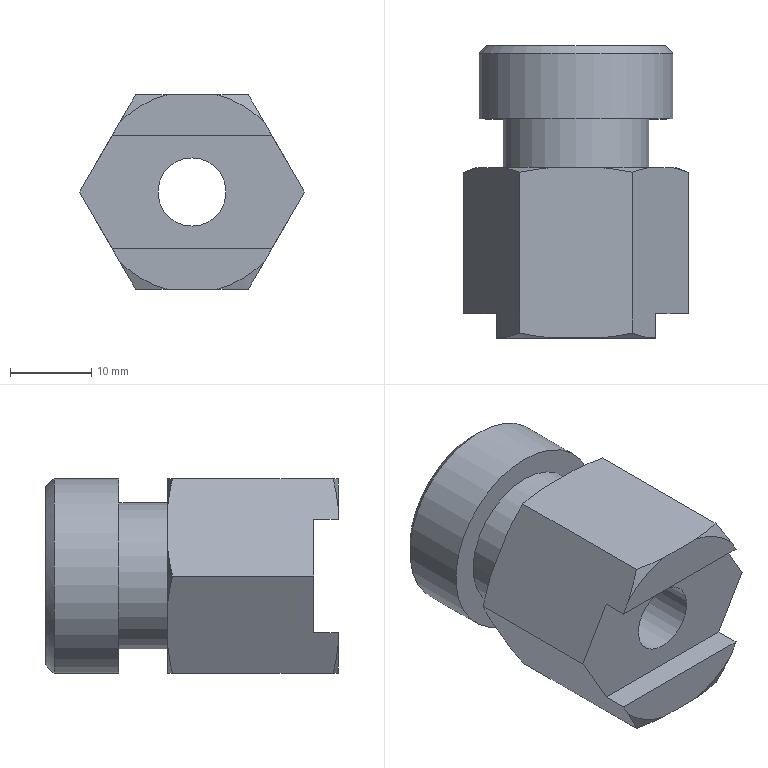Part | NX | 1 solid | 30 faces | box 27.713 x 36 x 24 mm | volume 12114 mm3 | plane 15 | cone 11 | cylinder 4 | commonest cylinder face diameters 8.4 x1 15 x1 18 x1 24 x1
STEP:
#1=CARTESIAN_POINT('',(6.928,-20.4,12.));
#2=VERTEX_POINT('',#1);
#3=CARTESIAN_POINT('',(6.928,-0.6,12.));
#4=VERTEX_POINT('',#3);
#5=CARTESIAN_POINT('',(6.928,-21.,12.));
#6=DIRECTION('',(0.,1.,0.));
#7=VECTOR('',#6,1000.);
#8=LINE('',#5,#7);
#9=EDGE_CURVE('',#2,#4,#8,.T.);
#10=ORIENTED_EDGE('',*,*,#9,.F.);
#11=CARTESIAN_POINT('',(8.919,-21.,8.552));
#12=VERTEX_POINT('',#11);
#13=CARTESIAN_POINT('',(6.928,-20.4,12.));
#14=CARTESIAN_POINT('',(7.585,-20.663,10.862));
#15=CARTESIAN_POINT('',(8.248,-20.872,9.715));
#16=CARTESIAN_POINT('',(8.919,-21.,8.552));
#17=B_SPLINE_CURVE_WITH_KNOTS('',3,(#13,#14,#15,#16),.UNSPECIFIED.,.F.,.F.,(4,4),(0.009948,0.01397),.UNSPECIFIED.);
#18=EDGE_CURVE('',#2,#12,#17,.T.);
#19=ORIENTED_EDGE('',*,*,#18,.T.);
#20=CARTESIAN_POINT('',(9.815,-21.,7.));
#21=VERTEX_POINT('',#20);
#22=CARTESIAN_POINT('',(6.928,-21.,12.));
#23=DIRECTION('',(0.5,0.,-0.866));
#24=VECTOR('',#23,1000.);
#25=LINE('',#22,#24);
#26=EDGE_CURVE('',#12,#21,#25,.T.);
#27=ORIENTED_EDGE('',*,*,#26,.T.);
#28=CARTESIAN_POINT('',(9.815,-18.,7.));
#29=VERTEX_POINT('',#28);
#30=CARTESIAN_POINT('',(9.815,-21.,7.));
#31=DIRECTION('',(0.,-1.,0.));
#32=VECTOR('',#31,1000.);
#33=LINE('',#30,#32);
#34=EDGE_CURVE('',#29,#21,#33,.T.);
#35=ORIENTED_EDGE('',*,*,#34,.F.);
#36=CARTESIAN_POINT('',(13.856,-18.,0.));
#37=VERTEX_POINT('',#36);
#38=CARTESIAN_POINT('',(6.928,-18.,12.));
#39=DIRECTION('',(-0.5,0.,0.866));
#40=VECTOR('',#39,1000.);
#41=LINE('',#38,#40);
#42=EDGE_CURVE('',#37,#29,#41,.T.);
#43=ORIENTED_EDGE('',*,*,#42,.F.);
#44=CARTESIAN_POINT('',(13.856,-0.6,0.));
#45=VERTEX_POINT('',#44);
#46=CARTESIAN_POINT('',(13.856,-21.,0.));
#47=DIRECTION('',(0.,1.,0.));
#48=VECTOR('',#47,1000.);
#49=LINE('',#46,#48);
#50=EDGE_CURVE('',#37,#45,#49,.T.);
#51=ORIENTED_EDGE('',*,*,#50,.T.);
#52=CARTESIAN_POINT('',(11.865,0.,3.448));
#53=VERTEX_POINT('',#52);
#54=CARTESIAN_POINT('',(13.856,-0.6,0.));
#55=CARTESIAN_POINT('',(13.2,-0.3373,1.138));
#56=CARTESIAN_POINT('',(12.537,-0.1281,2.285));
#57=CARTESIAN_POINT('',(11.865,0.,3.448));
#58=B_SPLINE_CURVE_WITH_KNOTS('',3,(#54,#55,#56,#57),.UNSPECIFIED.,.F.,.F.,(4,4),(0.009948,0.01397),.UNSPECIFIED.);
#59=EDGE_CURVE('',#45,#53,#58,.T.);
#60=ORIENTED_EDGE('',*,*,#59,.T.);
#61=CARTESIAN_POINT('',(8.919,0.,8.552));
#62=VERTEX_POINT('',#61);
#63=CARTESIAN_POINT('',(6.928,0.,12.));
#64=DIRECTION('',(0.5,0.,-0.866));
#65=VECTOR('',#64,1000.);
#66=LINE('',#63,#65);
#67=EDGE_CURVE('',#62,#53,#66,.T.);
#68=ORIENTED_EDGE('',*,*,#67,.F.);
#69=CARTESIAN_POINT('',(8.919,0.,8.552));
#70=CARTESIAN_POINT('',(8.249,-0.1279,9.713));
#71=CARTESIAN_POINT('',(7.586,-0.337,10.861));
#72=CARTESIAN_POINT('',(6.928,-0.6,12.));
#73=B_SPLINE_CURVE_WITH_KNOTS('',3,(#69,#70,#71,#72),.UNSPECIFIED.,.F.,.F.,(4,4),(0.01983,0.02389),.UNSPECIFIED.);
#74=EDGE_CURVE('',#62,#4,#73,.T.);
#75=ORIENTED_EDGE('',*,*,#74,.T.);
#76=EDGE_LOOP('',(#10,#19,#27,#35,#43,#51,#60,#68,#75));
#77=FACE_BOUND('',#76,.T.);
#78=CARTESIAN_POINT('',(6.928,-21.,12.));
#79=DIRECTION('',(0.866,0.,0.5));
#80=DIRECTION('',(0.5,0.,-0.866));
#81=AXIS2_PLACEMENT_3D('',#78,#79,#80);
#82=PLANE('',#81);
#83=ADVANCED_FACE('',(#77),#82,.T.);
#84=CARTESIAN_POINT('',(-6.928,-20.4,12.));
#85=VERTEX_POINT('',#84);
#86=CARTESIAN_POINT('',(-6.928,-0.6,12.));
#87=VERTEX_POINT('',#86);
#88=CARTESIAN_POINT('',(-6.928,-21.,12.));
#89=DIRECTION('',(0.,1.,0.));
#90=VECTOR('',#89,1000.);
#91=LINE('',#88,#90);
#92=EDGE_CURVE('',#85,#87,#91,.T.);
#93=ORIENTED_EDGE('',*,*,#92,.F.);
#94=CARTESIAN_POINT('',(-2.946,-21.,12.));
#95=VERTEX_POINT('',#94);
#96=CARTESIAN_POINT('',(-6.928,-20.4,12.));
#97=CARTESIAN_POINT('',(-5.613,-20.663,12.));
#98=CARTESIAN_POINT('',(-4.288,-20.872,12.));
#99=CARTESIAN_POINT('',(-2.946,-21.,12.));
#100=B_SPLINE_CURVE_WITH_KNOTS('',3,(#96,#97,#98,#99),.UNSPECIFIED.,.F.,.F.,(4,4),(0.008595,0.01262),.UNSPECIFIED.);
#101=EDGE_CURVE('',#85,#95,#100,.T.);
#102=ORIENTED_EDGE('',*,*,#101,.T.);
#103=CARTESIAN_POINT('',(2.946,-21.,12.));
#104=VERTEX_POINT('',#103);
#105=CARTESIAN_POINT('',(-6.928,-21.,12.));
#106=DIRECTION('',(1.,0.,0.));
#107=VECTOR('',#106,1000.);
#108=LINE('',#105,#107);
#109=EDGE_CURVE('',#95,#104,#108,.T.);
#110=ORIENTED_EDGE('',*,*,#109,.T.);
#111=CARTESIAN_POINT('',(2.946,-21.,12.));
#112=CARTESIAN_POINT('',(4.287,-20.872,12.));
#113=CARTESIAN_POINT('',(5.613,-20.663,12.));
#114=CARTESIAN_POINT('',(6.928,-20.4,12.));
#115=B_SPLINE_CURVE_WITH_KNOTS('',3,(#111,#112,#113,#114),.UNSPECIFIED.,.F.,.F.,(4,4),(0.01847,0.0225),.UNSPECIFIED.);
#116=EDGE_CURVE('',#104,#2,#115,.T.);
#117=ORIENTED_EDGE('',*,*,#116,.T.);
#118=ORIENTED_EDGE('',*,*,#9,.T.);
#119=CARTESIAN_POINT('',(2.946,0.,12.));
#120=VERTEX_POINT('',#119);
#121=CARTESIAN_POINT('',(6.928,-0.6,12.));
#122=CARTESIAN_POINT('',(5.613,-0.337,12.));
#123=CARTESIAN_POINT('',(4.288,-0.128,12.));
#124=CARTESIAN_POINT('',(2.946,0.,12.));
#125=B_SPLINE_CURVE_WITH_KNOTS('',3,(#121,#122,#123,#124),.UNSPECIFIED.,.F.,.F.,(4,4),(0.008595,0.01262),.UNSPECIFIED.);
#126=EDGE_CURVE('',#4,#120,#125,.T.);
#127=ORIENTED_EDGE('',*,*,#126,.T.);
#128=CARTESIAN_POINT('',(-2.946,0.,12.));
#129=VERTEX_POINT('',#128);
#130=CARTESIAN_POINT('',(-6.928,0.,12.));
#131=DIRECTION('',(1.,0.,0.));
#132=VECTOR('',#131,1000.);
#133=LINE('',#130,#132);
#134=EDGE_CURVE('',#129,#120,#133,.T.);
#135=ORIENTED_EDGE('',*,*,#134,.F.);
#136=CARTESIAN_POINT('',(-2.946,0.,12.));
#137=CARTESIAN_POINT('',(-4.287,-0.1279,12.));
#138=CARTESIAN_POINT('',(-5.613,-0.3369,12.));
#139=CARTESIAN_POINT('',(-6.928,-0.6,12.));
#140=B_SPLINE_CURVE_WITH_KNOTS('',3,(#136,#137,#138,#139),.UNSPECIFIED.,.F.,.F.,(4,4),(0.01847,0.0225),.UNSPECIFIED.);
#141=EDGE_CURVE('',#129,#87,#140,.T.);
#142=ORIENTED_EDGE('',*,*,#141,.T.);
#143=EDGE_LOOP('',(#93,#102,#110,#117,#118,#127,#135,#142));
#144=FACE_BOUND('',#143,.T.);
#145=CARTESIAN_POINT('',(-6.928,-21.,12.));
#146=DIRECTION('',(0.,0.,1.));
#147=DIRECTION('',(1.,0.,0.));
#148=AXIS2_PLACEMENT_3D('',#145,#146,#147);
#149=PLANE('',#148);
#150=ADVANCED_FACE('',(#144),#149,.T.);
#151=CARTESIAN_POINT('',(-9.815,-21.,7.));
#152=VERTEX_POINT('',#151);
#153=CARTESIAN_POINT('',(-8.919,-21.,8.552));
#154=VERTEX_POINT('',#153);
#155=CARTESIAN_POINT('',(-13.856,-21.,0.));
#156=DIRECTION('',(0.5,0.,0.866));
#157=VECTOR('',#156,1000.);
#158=LINE('',#155,#157);
#159=EDGE_CURVE('',#152,#154,#158,.T.);
#160=ORIENTED_EDGE('',*,*,#159,.T.);
#161=CARTESIAN_POINT('',(-8.919,-21.,8.552));
#162=CARTESIAN_POINT('',(-8.249,-20.872,9.713));
#163=CARTESIAN_POINT('',(-7.586,-20.663,10.861));
#164=CARTESIAN_POINT('',(-6.928,-20.4,12.));
#165=B_SPLINE_CURVE_WITH_KNOTS('',3,(#161,#162,#163,#164),.UNSPECIFIED.,.F.,.F.,(4,4),(0.01983,0.02389),.UNSPECIFIED.);
#166=EDGE_CURVE('',#154,#85,#165,.T.);
#167=ORIENTED_EDGE('',*,*,#166,.T.);
#168=ORIENTED_EDGE('',*,*,#92,.T.);
#169=CARTESIAN_POINT('',(-8.919,0.,8.552));
#170=VERTEX_POINT('',#169);
#171=CARTESIAN_POINT('',(-6.928,-0.6,12.));
#172=CARTESIAN_POINT('',(-7.585,-0.3373,10.862));
#173=CARTESIAN_POINT('',(-8.248,-0.1281,9.715));
#174=CARTESIAN_POINT('',(-8.919,0.,8.552));
#175=B_SPLINE_CURVE_WITH_KNOTS('',3,(#171,#172,#173,#174),.UNSPECIFIED.,.F.,.F.,(4,4),(0.009948,0.01397),.UNSPECIFIED.);
#176=EDGE_CURVE('',#87,#170,#175,.T.);
#177=ORIENTED_EDGE('',*,*,#176,.T.);
#178=CARTESIAN_POINT('',(-11.865,0.,3.448));
#179=VERTEX_POINT('',#178);
#180=CARTESIAN_POINT('',(-13.856,0.,0.));
#181=DIRECTION('',(0.5,0.,0.866));
#182=VECTOR('',#181,1000.);
#183=LINE('',#180,#182);
#184=EDGE_CURVE('',#179,#170,#183,.T.);
#185=ORIENTED_EDGE('',*,*,#184,.F.);
#186=CARTESIAN_POINT('',(-13.856,-0.6,0.));
#187=VERTEX_POINT('',#186);
#188=CARTESIAN_POINT('',(-11.865,0.,3.448));
#189=CARTESIAN_POINT('',(-12.536,-0.1279,2.287));
#190=CARTESIAN_POINT('',(-13.199,-0.337,1.139));
#191=CARTESIAN_POINT('',(-13.856,-0.6,0.));
#192=B_SPLINE_CURVE_WITH_KNOTS('',3,(#188,#189,#190,#191),.UNSPECIFIED.,.F.,.F.,(4,4),(0.01983,0.02389),.UNSPECIFIED.);
#193=EDGE_CURVE('',#179,#187,#192,.T.);
#194=ORIENTED_EDGE('',*,*,#193,.T.);
#195=CARTESIAN_POINT('',(-13.856,-18.,0.));
#196=VERTEX_POINT('',#195);
#197=CARTESIAN_POINT('',(-13.856,-21.,0.));
#198=DIRECTION('',(0.,1.,0.));
#199=VECTOR('',#198,1000.);
#200=LINE('',#197,#199);
#201=EDGE_CURVE('',#196,#187,#200,.T.);
#202=ORIENTED_EDGE('',*,*,#201,.F.);
#203=CARTESIAN_POINT('',(-9.815,-18.,7.));
#204=VERTEX_POINT('',#203);
#205=CARTESIAN_POINT('',(-13.856,-18.,0.));
#206=DIRECTION('',(-0.5,0.,-0.866));
#207=VECTOR('',#206,1000.);
#208=LINE('',#205,#207);
#209=EDGE_CURVE('',#204,#196,#208,.T.);
#210=ORIENTED_EDGE('',*,*,#209,.F.);
#211=CARTESIAN_POINT('',(-9.815,-21.,7.));
#212=DIRECTION('',(0.,1.,0.));
#213=VECTOR('',#212,1000.);
#214=LINE('',#211,#213);
#215=EDGE_CURVE('',#152,#204,#214,.T.);
#216=ORIENTED_EDGE('',*,*,#215,.F.);
#217=EDGE_LOOP('',(#160,#167,#168,#177,#185,#194,#202,#210,#216));
#218=FACE_BOUND('',#217,.T.);
#219=CARTESIAN_POINT('',(-13.856,-21.,0.));
#220=DIRECTION('',(-0.866,0.,0.5));
#221=DIRECTION('',(0.5,0.,0.866));
#222=AXIS2_PLACEMENT_3D('',#219,#220,#221);
#223=PLANE('',#222);
#224=ADVANCED_FACE('',(#218),#223,.T.);
#225=CARTESIAN_POINT('',(-6.928,-20.4,-12.));
#226=VERTEX_POINT('',#225);
#227=CARTESIAN_POINT('',(-6.928,-0.6,-12.));
#228=VERTEX_POINT('',#227);
#229=CARTESIAN_POINT('',(-6.928,-21.,-12.));
#230=DIRECTION('',(0.,1.,0.));
#231=VECTOR('',#230,1000.);
#232=LINE('',#229,#231);
#233=EDGE_CURVE('',#226,#228,#232,.T.);
#234=ORIENTED_EDGE('',*,*,#233,.F.);
#235=CARTESIAN_POINT('',(-8.919,-21.,-8.552));
#236=VERTEX_POINT('',#235);
#237=CARTESIAN_POINT('',(-6.928,-20.4,-12.));
#238=CARTESIAN_POINT('',(-7.585,-20.663,-10.862));
#239=CARTESIAN_POINT('',(-8.248,-20.872,-9.715));
#240=CARTESIAN_POINT('',(-8.919,-21.,-8.552));
#241=B_SPLINE_CURVE_WITH_KNOTS('',3,(#237,#238,#239,#240),.UNSPECIFIED.,.F.,.F.,(4,4),(0.009948,0.01397),.UNSPECIFIED.);
#242=EDGE_CURVE('',#226,#236,#241,.T.);
#243=ORIENTED_EDGE('',*,*,#242,.T.);
#244=CARTESIAN_POINT('',(-9.815,-21.,-7.));
#245=VERTEX_POINT('',#244);
#246=CARTESIAN_POINT('',(-6.928,-21.,-12.));
#247=DIRECTION('',(-0.5,0.,0.866));
#248=VECTOR('',#247,1000.);
#249=LINE('',#246,#248);
#250=EDGE_CURVE('',#236,#245,#249,.T.);
#251=ORIENTED_EDGE('',*,*,#250,.T.);
#252=CARTESIAN_POINT('',(-9.815,-18.,-7.));
#253=VERTEX_POINT('',#252);
#254=CARTESIAN_POINT('',(-9.815,-21.,-7.));
#255=DIRECTION('',(0.,-1.,0.));
#256=VECTOR('',#255,1000.);
#257=LINE('',#254,#256);
#258=EDGE_CURVE('',#253,#245,#257,.T.);
#259=ORIENTED_EDGE('',*,*,#258,.F.);
#260=CARTESIAN_POINT('',(-6.928,-18.,-12.));
#261=DIRECTION('',(0.5,0.,-0.866));
#262=VECTOR('',#261,1000.);
#263=LINE('',#260,#262);
#264=EDGE_CURVE('',#196,#253,#263,.T.);
#265=ORIENTED_EDGE('',*,*,#264,.F.);
#266=ORIENTED_EDGE('',*,*,#201,.T.);
#267=CARTESIAN_POINT('',(-11.865,0.,-3.448));
#268=VERTEX_POINT('',#267);
#269=CARTESIAN_POINT('',(-13.856,-0.6,0.));
#270=CARTESIAN_POINT('',(-13.2,-0.3373,-1.138));
#271=CARTESIAN_POINT('',(-12.537,-0.1281,-2.285));
#272=CARTESIAN_POINT('',(-11.865,0.,-3.448));
#273=B_SPLINE_CURVE_WITH_KNOTS('',3,(#269,#270,#271,#272),.UNSPECIFIED.,.F.,.F.,(4,4),(0.009948,0.01397),.UNSPECIFIED.);
#274=EDGE_CURVE('',#187,#268,#273,.T.);
#275=ORIENTED_EDGE('',*,*,#274,.T.);
#276=CARTESIAN_POINT('',(-8.919,0.,-8.552));
#277=VERTEX_POINT('',#276);
#278=CARTESIAN_POINT('',(-6.928,0.,-12.));
#279=DIRECTION('',(-0.5,0.,0.866));
#280=VECTOR('',#279,1000.);
#281=LINE('',#278,#280);
#282=EDGE_CURVE('',#277,#268,#281,.T.);
#283=ORIENTED_EDGE('',*,*,#282,.F.);
#284=CARTESIAN_POINT('',(-8.919,0.,-8.552));
#285=CARTESIAN_POINT('',(-8.249,-0.1279,-9.713));
#286=CARTESIAN_POINT('',(-7.586,-0.337,-10.861));
#287=CARTESIAN_POINT('',(-6.928,-0.6,-12.));
#288=B_SPLINE_CURVE_WITH_KNOTS('',3,(#284,#285,#286,#287),.UNSPECIFIED.,.F.,.F.,(4,4),(0.01983,0.02389),.UNSPECIFIED.);
#289=EDGE_CURVE('',#277,#228,#288,.T.);
#290=ORIENTED_EDGE('',*,*,#289,.T.);
#291=EDGE_LOOP('',(#234,#243,#251,#259,#265,#266,#275,#283,#290));
#292=FACE_BOUND('',#291,.T.);
#293=CARTESIAN_POINT('',(-6.928,-21.,-12.));
#294=DIRECTION('',(-0.866,0.,-0.5));
#295=DIRECTION('',(-0.5,0.,0.866));
#296=AXIS2_PLACEMENT_3D('',#293,#294,#295);
#297=PLANE('',#296);
#298=ADVANCED_FACE('',(#292),#297,.T.);
#299=CARTESIAN_POINT('',(6.928,-20.4,-12.));
#300=VERTEX_POINT('',#299);
#301=CARTESIAN_POINT('',(6.928,-0.6,-12.));
#302=VERTEX_POINT('',#301);
#303=CARTESIAN_POINT('',(6.928,-21.,-12.));
#304=DIRECTION('',(0.,1.,0.));
#305=VECTOR('',#304,1000.);
#306=LINE('',#303,#305);
#307=EDGE_CURVE('',#300,#302,#306,.T.);
#308=ORIENTED_EDGE('',*,*,#307,.F.);
#309=CARTESIAN_POINT('',(2.946,-21.,-12.));
#310=VERTEX_POINT('',#309);
#311=CARTESIAN_POINT('',(6.928,-20.4,-12.));
#312=CARTESIAN_POINT('',(5.613,-20.663,-12.));
#313=CARTESIAN_POINT('',(4.288,-20.872,-12.));
#314=CARTESIAN_POINT('',(2.946,-21.,-12.));
#315=B_SPLINE_CURVE_WITH_KNOTS('',3,(#311,#312,#313,#314),.UNSPECIFIED.,.F.,.F.,(4,4),(0.008595,0.01262),.UNSPECIFIED.);
#316=EDGE_CURVE('',#300,#310,#315,.T.);
#317=ORIENTED_EDGE('',*,*,#316,.T.);
#318=CARTESIAN_POINT('',(-2.946,-21.,-12.));
#319=VERTEX_POINT('',#318);
#320=CARTESIAN_POINT('',(6.928,-21.,-12.));
#321=DIRECTION('',(-1.,0.,0.));
#322=VECTOR('',#321,1000.);
#323=LINE('',#320,#322);
#324=EDGE_CURVE('',#310,#319,#323,.T.);
#325=ORIENTED_EDGE('',*,*,#324,.T.);
#326=CARTESIAN_POINT('',(-2.946,-21.,-12.));
#327=CARTESIAN_POINT('',(-4.287,-20.872,-12.));
#328=CARTESIAN_POINT('',(-5.613,-20.663,-12.));
#329=CARTESIAN_POINT('',(-6.928,-20.4,-12.));
#330=B_SPLINE_CURVE_WITH_KNOTS('',3,(#326,#327,#328,#329),.UNSPECIFIED.,.F.,.F.,(4,4),(0.01847,0.0225),.UNSPECIFIED.);
#331=EDGE_CURVE('',#319,#226,#330,.T.);
#332=ORIENTED_EDGE('',*,*,#331,.T.);
#333=ORIENTED_EDGE('',*,*,#233,.T.);
#334=CARTESIAN_POINT('',(-2.946,0.,-12.));
#335=VERTEX_POINT('',#334);
#336=CARTESIAN_POINT('',(-6.928,-0.6,-12.));
#337=CARTESIAN_POINT('',(-5.613,-0.337,-12.));
#338=CARTESIAN_POINT('',(-4.288,-0.128,-12.));
#339=CARTESIAN_POINT('',(-2.946,0.,-12.));
#340=B_SPLINE_CURVE_WITH_KNOTS('',3,(#336,#337,#338,#339),.UNSPECIFIED.,.F.,.F.,(4,4),(0.008595,0.01262),.UNSPECIFIED.);
#341=EDGE_CURVE('',#228,#335,#340,.T.);
#342=ORIENTED_EDGE('',*,*,#341,.T.);
#343=CARTESIAN_POINT('',(2.946,0.,-12.));
#344=VERTEX_POINT('',#343);
#345=CARTESIAN_POINT('',(6.928,0.,-12.));
#346=DIRECTION('',(-1.,0.,0.));
#347=VECTOR('',#346,1000.);
#348=LINE('',#345,#347);
#349=EDGE_CURVE('',#344,#335,#348,.T.);
#350=ORIENTED_EDGE('',*,*,#349,.F.);
#351=CARTESIAN_POINT('',(2.946,0.,-12.));
#352=CARTESIAN_POINT('',(4.287,-0.1279,-12.));
#353=CARTESIAN_POINT('',(5.613,-0.3369,-12.));
#354=CARTESIAN_POINT('',(6.928,-0.6,-12.));
#355=B_SPLINE_CURVE_WITH_KNOTS('',3,(#351,#352,#353,#354),.UNSPECIFIED.,.F.,.F.,(4,4),(0.01847,0.0225),.UNSPECIFIED.);
#356=EDGE_CURVE('',#344,#302,#355,.T.);
#357=ORIENTED_EDGE('',*,*,#356,.T.);
#358=EDGE_LOOP('',(#308,#317,#325,#332,#333,#342,#350,#357));
#359=FACE_BOUND('',#358,.T.);
#360=CARTESIAN_POINT('',(6.928,-21.,-12.));
#361=DIRECTION('',(0.,0.,-1.));
#362=DIRECTION('',(-1.,0.,0.));
#363=AXIS2_PLACEMENT_3D('',#360,#361,#362);
#364=PLANE('',#363);
#365=ADVANCED_FACE('',(#359),#364,.T.);
#366=CARTESIAN_POINT('',(9.815,-21.,-7.));
#367=VERTEX_POINT('',#366);
#368=CARTESIAN_POINT('',(8.919,-21.,-8.552));
#369=VERTEX_POINT('',#368);
#370=CARTESIAN_POINT('',(13.856,-21.,0.));
#371=DIRECTION('',(-0.5,0.,-0.866));
#372=VECTOR('',#371,1000.);
#373=LINE('',#370,#372);
#374=EDGE_CURVE('',#367,#369,#373,.T.);
#375=ORIENTED_EDGE('',*,*,#374,.T.);
#376=CARTESIAN_POINT('',(8.919,-21.,-8.552));
#377=CARTESIAN_POINT('',(8.249,-20.872,-9.713));
#378=CARTESIAN_POINT('',(7.586,-20.663,-10.861));
#379=CARTESIAN_POINT('',(6.928,-20.4,-12.));
#380=B_SPLINE_CURVE_WITH_KNOTS('',3,(#376,#377,#378,#379),.UNSPECIFIED.,.F.,.F.,(4,4),(0.01983,0.02389),.UNSPECIFIED.);
#381=EDGE_CURVE('',#369,#300,#380,.T.);
#382=ORIENTED_EDGE('',*,*,#381,.T.);
#383=ORIENTED_EDGE('',*,*,#307,.T.);
#384=CARTESIAN_POINT('',(8.919,0.,-8.552));
#385=VERTEX_POINT('',#384);
#386=CARTESIAN_POINT('',(6.928,-0.6,-12.));
#387=CARTESIAN_POINT('',(7.585,-0.3373,-10.862));
#388=CARTESIAN_POINT('',(8.248,-0.1281,-9.715));
#389=CARTESIAN_POINT('',(8.919,0.,-8.552));
#390=B_SPLINE_CURVE_WITH_KNOTS('',3,(#386,#387,#388,#389),.UNSPECIFIED.,.F.,.F.,(4,4),(0.009948,0.01397),.UNSPECIFIED.);
#391=EDGE_CURVE('',#302,#385,#390,.T.);
#392=ORIENTED_EDGE('',*,*,#391,.T.);
#393=CARTESIAN_POINT('',(11.865,0.,-3.448));
#394=VERTEX_POINT('',#393);
#395=CARTESIAN_POINT('',(13.856,0.,0.));
#396=DIRECTION('',(-0.5,0.,-0.866));
#397=VECTOR('',#396,1000.);
#398=LINE('',#395,#397);
#399=EDGE_CURVE('',#394,#385,#398,.T.);
#400=ORIENTED_EDGE('',*,*,#399,.F.);
#401=CARTESIAN_POINT('',(11.865,0.,-3.448));
#402=CARTESIAN_POINT('',(12.536,-0.1279,-2.287));
#403=CARTESIAN_POINT('',(13.199,-0.337,-1.139));
#404=CARTESIAN_POINT('',(13.856,-0.6,0.));
#405=B_SPLINE_CURVE_WITH_KNOTS('',3,(#401,#402,#403,#404),.UNSPECIFIED.,.F.,.F.,(4,4),(0.01983,0.02389),.UNSPECIFIED.);
#406=EDGE_CURVE('',#394,#45,#405,.T.);
#407=ORIENTED_EDGE('',*,*,#406,.T.);
#408=ORIENTED_EDGE('',*,*,#50,.F.);
#409=CARTESIAN_POINT('',(9.815,-18.,-7.));
#410=VERTEX_POINT('',#409);
#411=CARTESIAN_POINT('',(13.856,-18.,0.));
#412=DIRECTION('',(0.5,0.,0.866));
#413=VECTOR('',#412,1000.);
#414=LINE('',#411,#413);
#415=EDGE_CURVE('',#410,#37,#414,.T.);
#416=ORIENTED_EDGE('',*,*,#415,.F.);
#417=CARTESIAN_POINT('',(9.815,-21.,-7.));
#418=DIRECTION('',(0.,1.,0.));
#419=VECTOR('',#418,1000.);
#420=LINE('',#417,#419);
#421=EDGE_CURVE('',#367,#410,#420,.T.);
#422=ORIENTED_EDGE('',*,*,#421,.F.);
#423=EDGE_LOOP('',(#375,#382,#383,#392,#400,#407,#408,#416,#422));
#424=FACE_BOUND('',#423,.T.);
#425=CARTESIAN_POINT('',(13.856,-21.,0.));
#426=DIRECTION('',(0.866,0.,-0.5));
#427=DIRECTION('',(-0.5,0.,-0.866));
#428=AXIS2_PLACEMENT_3D('',#425,#426,#427);
#429=PLANE('',#428);
#430=ADVANCED_FACE('',(#424),#429,.T.);
#431=CARTESIAN_POINT('',(0.,-21.,0.));
#432=DIRECTION('',(0.,1.,0.));
#433=DIRECTION('',(0.,0.,1.));
#434=AXIS2_PLACEMENT_3D('',#431,#432,#433);
#435=CIRCLE('',#434,12.356);
#436=EDGE_CURVE('',#104,#12,#435,.T.);
#437=ORIENTED_EDGE('',*,*,#436,.F.);
#438=ORIENTED_EDGE('',*,*,#109,.F.);
#439=CARTESIAN_POINT('',(0.,-21.,0.));
#440=DIRECTION('',(0.,1.,0.));
#441=DIRECTION('',(0.,0.,1.));
#442=AXIS2_PLACEMENT_3D('',#439,#440,#441);
#443=CIRCLE('',#442,12.356);
#444=EDGE_CURVE('',#154,#95,#443,.T.);
#445=ORIENTED_EDGE('',*,*,#444,.F.);
#446=ORIENTED_EDGE('',*,*,#159,.F.);
#447=CARTESIAN_POINT('',(0.,-21.,7.));
#448=DIRECTION('',(1.,0.,0.));
#449=VECTOR('',#448,1000.);
#450=LINE('',#447,#449);
#451=EDGE_CURVE('',#152,#21,#450,.T.);
#452=ORIENTED_EDGE('',*,*,#451,.T.);
#453=ORIENTED_EDGE('',*,*,#26,.F.);
#454=EDGE_LOOP('',(#437,#438,#445,#446,#452,#453));
#455=FACE_BOUND('',#454,.T.);
#456=CARTESIAN_POINT('',(0.,-21.,0.));
#457=DIRECTION('',(0.,1.,0.));
#458=DIRECTION('',(0.,0.,1.));
#459=AXIS2_PLACEMENT_3D('',#456,#457,#458);
#460=PLANE('',#459);
#461=ADVANCED_FACE('',(#455),#460,.F.);
#462=CARTESIAN_POINT('',(0.,-21.,0.));
#463=DIRECTION('',(0.,1.,0.));
#464=DIRECTION('',(0.,0.,1.));
#465=AXIS2_PLACEMENT_3D('',#462,#463,#464);
#466=CIRCLE('',#465,12.356);
#467=EDGE_CURVE('',#369,#310,#466,.T.);
#468=ORIENTED_EDGE('',*,*,#467,.F.);
#469=ORIENTED_EDGE('',*,*,#374,.F.);
#470=CARTESIAN_POINT('',(0.,-21.,-7.));
#471=DIRECTION('',(-1.,0.,0.));
#472=VECTOR('',#471,1000.);
#473=LINE('',#470,#472);
#474=EDGE_CURVE('',#367,#245,#473,.T.);
#475=ORIENTED_EDGE('',*,*,#474,.T.);
#476=ORIENTED_EDGE('',*,*,#250,.F.);
#477=CARTESIAN_POINT('',(0.,-21.,0.));
#478=DIRECTION('',(0.,1.,0.));
#479=DIRECTION('',(0.,0.,1.));
#480=AXIS2_PLACEMENT_3D('',#477,#478,#479);
#481=CIRCLE('',#480,12.356);
#482=EDGE_CURVE('',#319,#236,#481,.T.);
#483=ORIENTED_EDGE('',*,*,#482,.F.);
#484=ORIENTED_EDGE('',*,*,#324,.F.);
#485=EDGE_LOOP('',(#468,#469,#475,#476,#483,#484));
#486=FACE_BOUND('',#485,.T.);
#487=CARTESIAN_POINT('',(0.,-21.,0.));
#488=DIRECTION('',(0.,1.,0.));
#489=DIRECTION('',(0.,0.,1.));
#490=AXIS2_PLACEMENT_3D('',#487,#488,#489);
#491=PLANE('',#490);
#492=ADVANCED_FACE('',(#486),#491,.F.);
#493=CARTESIAN_POINT('',(0.,0.,9.));
#494=VERTEX_POINT('',#493);
#495=CARTESIAN_POINT('',(0.,0.,0.));
#496=DIRECTION('',(0.,1.,0.));
#497=DIRECTION('',(0.,0.,1.));
#498=AXIS2_PLACEMENT_3D('',#495,#496,#497);
#499=CIRCLE('',#498,9.);
#500=EDGE_CURVE('',#494,#494,#499,.T.);
#501=ORIENTED_EDGE('',*,*,#500,.F.);
#502=EDGE_LOOP('',(#501));
#503=FACE_BOUND('',#502,.T.);
#504=ORIENTED_EDGE('',*,*,#134,.T.);
#505=CARTESIAN_POINT('',(0.,0.,0.));
#506=DIRECTION('',(0.,1.,0.));
#507=DIRECTION('',(0.,0.,1.));
#508=AXIS2_PLACEMENT_3D('',#505,#506,#507);
#509=CIRCLE('',#508,12.356);
#510=EDGE_CURVE('',#120,#62,#509,.T.);
#511=ORIENTED_EDGE('',*,*,#510,.T.);
#512=ORIENTED_EDGE('',*,*,#67,.T.);
#513=CARTESIAN_POINT('',(0.,0.,0.));
#514=DIRECTION('',(0.,1.,0.));
#515=DIRECTION('',(0.,0.,1.));
#516=AXIS2_PLACEMENT_3D('',#513,#514,#515);
#517=CIRCLE('',#516,12.356);
#518=EDGE_CURVE('',#53,#394,#517,.T.);
#519=ORIENTED_EDGE('',*,*,#518,.T.);
#520=ORIENTED_EDGE('',*,*,#399,.T.);
#521=CARTESIAN_POINT('',(0.,0.,0.));
#522=DIRECTION('',(0.,1.,0.));
#523=DIRECTION('',(0.,0.,1.));
#524=AXIS2_PLACEMENT_3D('',#521,#522,#523);
#525=CIRCLE('',#524,12.356);
#526=EDGE_CURVE('',#385,#344,#525,.T.);
#527=ORIENTED_EDGE('',*,*,#526,.T.);
#528=ORIENTED_EDGE('',*,*,#349,.T.);
#529=CARTESIAN_POINT('',(0.,0.,0.));
#530=DIRECTION('',(0.,1.,0.));
#531=DIRECTION('',(0.,0.,1.));
#532=AXIS2_PLACEMENT_3D('',#529,#530,#531);
#533=CIRCLE('',#532,12.356);
#534=EDGE_CURVE('',#335,#277,#533,.T.);
#535=ORIENTED_EDGE('',*,*,#534,.T.);
#536=ORIENTED_EDGE('',*,*,#282,.T.);
#537=CARTESIAN_POINT('',(0.,0.,0.));
#538=DIRECTION('',(0.,1.,0.));
#539=DIRECTION('',(0.,0.,1.));
#540=AXIS2_PLACEMENT_3D('',#537,#538,#539);
#541=CIRCLE('',#540,12.356);
#542=EDGE_CURVE('',#268,#179,#541,.T.);
#543=ORIENTED_EDGE('',*,*,#542,.T.);
#544=ORIENTED_EDGE('',*,*,#184,.T.);
#545=CARTESIAN_POINT('',(0.,0.,0.));
#546=DIRECTION('',(0.,1.,0.));
#547=DIRECTION('',(0.,0.,1.));
#548=AXIS2_PLACEMENT_3D('',#545,#546,#547);
#549=CIRCLE('',#548,12.356);
#550=EDGE_CURVE('',#170,#129,#549,.T.);
#551=ORIENTED_EDGE('',*,*,#550,.T.);
#552=EDGE_LOOP('',(#504,#511,#512,#519,#520,#527,#528,#535,#536,#543,#544,#551));
#553=FACE_BOUND('',#552,.T.);
#554=CARTESIAN_POINT('',(0.,0.,0.));
#555=DIRECTION('',(0.,1.,0.));
#556=DIRECTION('',(0.,0.,1.));
#557=AXIS2_PLACEMENT_3D('',#554,#555,#556);
#558=PLANE('',#557);
#559=ADVANCED_FACE('',(#503,#553),#558,.T.);
#560=CARTESIAN_POINT('',(0.,6.,9.));
#561=VERTEX_POINT('',#560);
#562=CARTESIAN_POINT('',(0.,6.,0.));
#563=DIRECTION('',(0.,1.,0.));
#564=DIRECTION('',(0.,0.,1.));
#565=AXIS2_PLACEMENT_3D('',#562,#563,#564);
#566=CIRCLE('',#565,9.);
#567=EDGE_CURVE('',#561,#561,#566,.T.);
#568=ORIENTED_EDGE('',*,*,#567,.T.);
#569=EDGE_LOOP('',(#568));
#570=FACE_BOUND('',#569,.T.);
#571=CARTESIAN_POINT('',(0.,6.,12.));
#572=VERTEX_POINT('',#571);
#573=CARTESIAN_POINT('',(0.,6.,0.));
#574=DIRECTION('',(0.,1.,0.));
#575=DIRECTION('',(0.,0.,1.));
#576=AXIS2_PLACEMENT_3D('',#573,#574,#575);
#577=CIRCLE('',#576,12.);
#578=EDGE_CURVE('',#572,#572,#577,.T.);
#579=ORIENTED_EDGE('',*,*,#578,.F.);
#580=EDGE_LOOP('',(#579));
#581=FACE_BOUND('',#580,.T.);
#582=CARTESIAN_POINT('',(0.,6.,0.));
#583=DIRECTION('',(0.,1.,0.));
#584=DIRECTION('',(0.,0.,1.));
#585=AXIS2_PLACEMENT_3D('',#582,#583,#584);
#586=PLANE('',#585);
#587=ADVANCED_FACE('',(#570,#581),#586,.F.);
#588=CARTESIAN_POINT('',(0.,15.,11.));
#589=VERTEX_POINT('',#588);
#590=CARTESIAN_POINT('',(0.,15.,0.));
#591=DIRECTION('',(0.,1.,0.));
#592=DIRECTION('',(0.,0.,1.));
#593=AXIS2_PLACEMENT_3D('',#590,#591,#592);
#594=CIRCLE('',#593,11.);
#595=EDGE_CURVE('',#589,#589,#594,.T.);
#596=ORIENTED_EDGE('',*,*,#595,.T.);
#597=EDGE_LOOP('',(#596));
#598=FACE_BOUND('',#597,.T.);
#599=CARTESIAN_POINT('',(0.,15.,7.5));
#600=VERTEX_POINT('',#599);
#601=CARTESIAN_POINT('',(0.,15.,0.));
#602=DIRECTION('',(0.,1.,0.));
#603=DIRECTION('',(0.,0.,1.));
#604=AXIS2_PLACEMENT_3D('',#601,#602,#603);
#605=CIRCLE('',#604,7.5);
#606=EDGE_CURVE('',#600,#600,#605,.T.);
#607=ORIENTED_EDGE('',*,*,#606,.F.);
#608=EDGE_LOOP('',(#607));
#609=FACE_BOUND('',#608,.T.);
#610=CARTESIAN_POINT('',(0.,15.,0.));
#611=DIRECTION('',(0.,1.,0.));
#612=DIRECTION('',(0.,0.,1.));
#613=AXIS2_PLACEMENT_3D('',#610,#611,#612);
#614=PLANE('',#613);
#615=ADVANCED_FACE('',(#598,#609),#614,.T.);
#616=ORIENTED_EDGE('',*,*,#34,.T.);
#617=ORIENTED_EDGE('',*,*,#451,.F.);
#618=ORIENTED_EDGE('',*,*,#215,.T.);
#619=CARTESIAN_POINT('',(-15.,-18.,7.));
#620=DIRECTION('',(-1.,0.,0.));
#621=VECTOR('',#620,1000.);
#622=LINE('',#619,#621);
#623=EDGE_CURVE('',#29,#204,#622,.T.);
#624=ORIENTED_EDGE('',*,*,#623,.F.);
#625=EDGE_LOOP('',(#616,#617,#618,#624));
#626=FACE_BOUND('',#625,.T.);
#627=CARTESIAN_POINT('',(-15.,-18.,7.));
#628=DIRECTION('',(0.,0.,1.));
#629=DIRECTION('',(1.,0.,0.));
#630=AXIS2_PLACEMENT_3D('',#627,#628,#629);
#631=PLANE('',#630);
#632=ADVANCED_FACE('',(#626),#631,.F.);
#633=ORIENTED_EDGE('',*,*,#258,.T.);
#634=ORIENTED_EDGE('',*,*,#474,.F.);
#635=ORIENTED_EDGE('',*,*,#421,.T.);
#636=CARTESIAN_POINT('',(-15.,-18.,-7.));
#637=DIRECTION('',(1.,0.,0.));
#638=VECTOR('',#637,1000.);
#639=LINE('',#636,#638);
#640=EDGE_CURVE('',#253,#410,#639,.T.);
#641=ORIENTED_EDGE('',*,*,#640,.F.);
#642=EDGE_LOOP('',(#633,#634,#635,#641));
#643=FACE_BOUND('',#642,.T.);
#644=CARTESIAN_POINT('',(-15.,-18.,-7.));
#645=DIRECTION('',(0.,0.,-1.));
#646=DIRECTION('',(-1.,0.,0.));
#647=AXIS2_PLACEMENT_3D('',#644,#645,#646);
#648=PLANE('',#647);
#649=ADVANCED_FACE('',(#643),#648,.F.);
#650=CARTESIAN_POINT('',(0.,-18.,4.2));
#651=VERTEX_POINT('',#650);
#652=CARTESIAN_POINT('',(0.,-18.,0.));
#653=DIRECTION('',(0.,1.,0.));
#654=DIRECTION('',(0.,0.,1.));
#655=AXIS2_PLACEMENT_3D('',#652,#653,#654);
#656=CIRCLE('',#655,4.2);
#657=EDGE_CURVE('',#651,#651,#656,.T.);
#658=ORIENTED_EDGE('',*,*,#657,.T.);
#659=EDGE_LOOP('',(#658));
#660=FACE_BOUND('',#659,.T.);
#661=ORIENTED_EDGE('',*,*,#209,.T.);
#662=ORIENTED_EDGE('',*,*,#264,.T.);
#663=ORIENTED_EDGE('',*,*,#640,.T.);
#664=ORIENTED_EDGE('',*,*,#415,.T.);
#665=ORIENTED_EDGE('',*,*,#42,.T.);
#666=ORIENTED_EDGE('',*,*,#623,.T.);
#667=EDGE_LOOP('',(#661,#662,#663,#664,#665,#666));
#668=FACE_BOUND('',#667,.T.);
#669=CARTESIAN_POINT('',(0.,-18.,0.));
#670=DIRECTION('',(0.,1.,0.));
#671=DIRECTION('',(0.,0.,1.));
#672=AXIS2_PLACEMENT_3D('',#669,#670,#671);
#673=PLANE('',#672);
#674=ADVANCED_FACE('',(#660,#668),#673,.F.);
#675=ORIENTED_EDGE('',*,*,#567,.F.);
#676=EDGE_LOOP('',(#675));
#677=FACE_BOUND('',#676,.T.);
#678=ORIENTED_EDGE('',*,*,#500,.T.);
#679=EDGE_LOOP('',(#678));
#680=FACE_BOUND('',#679,.T.);
#681=CARTESIAN_POINT('',(0.,6.,0.));
#682=DIRECTION('',(0.,-1.,0.));
#683=DIRECTION('',(0.,0.,-1.));
#684=AXIS2_PLACEMENT_3D('',#681,#682,#683);
#685=CYLINDRICAL_SURFACE('',#684,9.);
#686=ADVANCED_FACE('',(#677,#680),#685,.T.);
#687=CARTESIAN_POINT('',(0.,6.,4.2));
#688=VERTEX_POINT('',#687);
#689=CARTESIAN_POINT('',(0.,6.,0.));
#690=DIRECTION('',(0.,1.,0.));
#691=DIRECTION('',(0.,0.,1.));
#692=AXIS2_PLACEMENT_3D('',#689,#690,#691);
#693=CIRCLE('',#692,4.2);
#694=EDGE_CURVE('',#688,#688,#693,.T.);
#695=ORIENTED_EDGE('',*,*,#694,.T.);
#696=EDGE_LOOP('',(#695));
#697=FACE_BOUND('',#696,.T.);
#698=ORIENTED_EDGE('',*,*,#657,.F.);
#699=EDGE_LOOP('',(#698));
#700=FACE_BOUND('',#699,.T.);
#701=CARTESIAN_POINT('',(0.,15.,0.));
#702=DIRECTION('',(0.,1.,0.));
#703=DIRECTION('',(0.,0.,1.));
#704=AXIS2_PLACEMENT_3D('',#701,#702,#703);
#705=CYLINDRICAL_SURFACE('',#704,4.2);
#706=ADVANCED_FACE('',(#697,#700),#705,.F.);
#707=ORIENTED_EDGE('',*,*,#694,.F.);
#708=EDGE_LOOP('',(#707));
#709=FACE_BOUND('',#708,.T.);
#710=CARTESIAN_POINT('',(0.,6.,7.5));
#711=VERTEX_POINT('',#710);
#712=CARTESIAN_POINT('',(0.,6.,0.));
#713=DIRECTION('',(0.,1.,0.));
#714=DIRECTION('',(0.,0.,1.));
#715=AXIS2_PLACEMENT_3D('',#712,#713,#714);
#716=CIRCLE('',#715,7.5);
#717=EDGE_CURVE('',#711,#711,#716,.T.);
#718=ORIENTED_EDGE('',*,*,#717,.T.);
#719=EDGE_LOOP('',(#718));
#720=FACE_BOUND('',#719,.T.);
#721=CARTESIAN_POINT('',(4.2,6.,0.));
#722=DIRECTION('',(0.,-1.,0.));
#723=DIRECTION('',(0.,0.,-1.));
#724=AXIS2_PLACEMENT_3D('',#721,#722,#723);
#725=PLANE('',#724);
#726=ADVANCED_FACE('',(#709,#720),#725,.F.);
#727=ORIENTED_EDGE('',*,*,#717,.F.);
#728=EDGE_LOOP('',(#727));
#729=FACE_BOUND('',#728,.T.);
#730=ORIENTED_EDGE('',*,*,#606,.T.);
#731=EDGE_LOOP('',(#730));
#732=FACE_BOUND('',#731,.T.);
#733=CARTESIAN_POINT('',(0.,15.,0.));
#734=DIRECTION('',(0.,1.,0.));
#735=DIRECTION('',(0.,0.,1.));
#736=AXIS2_PLACEMENT_3D('',#733,#734,#735);
#737=CYLINDRICAL_SURFACE('',#736,7.5);
#738=ADVANCED_FACE('',(#729,#732),#737,.F.);
#739=CARTESIAN_POINT('',(0.,14.,12.));
#740=VERTEX_POINT('',#739);
#741=CARTESIAN_POINT('',(0.,14.,0.));
#742=DIRECTION('',(0.,1.,0.));
#743=DIRECTION('',(0.,0.,1.));
#744=AXIS2_PLACEMENT_3D('',#741,#742,#743);
#745=CIRCLE('',#744,12.);
#746=EDGE_CURVE('',#740,#740,#745,.F.);
#747=ORIENTED_EDGE('',*,*,#746,.T.);
#748=EDGE_LOOP('',(#747));
#749=FACE_BOUND('',#748,.T.);
#750=ORIENTED_EDGE('',*,*,#578,.T.);
#751=EDGE_LOOP('',(#750));
#752=FACE_BOUND('',#751,.T.);
#753=CARTESIAN_POINT('',(0.,5.,0.));
#754=DIRECTION('',(0.,1.,0.));
#755=DIRECTION('',(0.,0.,1.));
#756=AXIS2_PLACEMENT_3D('',#753,#754,#755);
#757=CYLINDRICAL_SURFACE('',#756,12.);
#758=ADVANCED_FACE('',(#749,#752),#757,.T.);
#759=ORIENTED_EDGE('',*,*,#746,.F.);
#760=EDGE_LOOP('',(#759));
#761=FACE_BOUND('',#760,.T.);
#762=ORIENTED_EDGE('',*,*,#595,.F.);
#763=EDGE_LOOP('',(#762));
#764=FACE_BOUND('',#763,.T.);
#765=CARTESIAN_POINT('',(0.,15.,0.));
#766=DIRECTION('',(0.,-1.,0.));
#767=DIRECTION('',(0.,0.,-1.));
#768=AXIS2_PLACEMENT_3D('',#765,#766,#767);
#769=CONICAL_SURFACE('',#768,11.,0.7854);
#770=ADVANCED_FACE('',(#761,#764),#769,.T.);
#771=ORIENTED_EDGE('',*,*,#550,.F.);
#772=ORIENTED_EDGE('',*,*,#176,.F.);
#773=ORIENTED_EDGE('',*,*,#141,.F.);
#774=EDGE_LOOP('',(#771,#772,#773));
#775=FACE_BOUND('',#774,.T.);
#776=CARTESIAN_POINT('',(0.,0.,0.));
#777=DIRECTION('',(0.,-1.,0.));
#778=DIRECTION('',(0.,0.,-1.));
#779=AXIS2_PLACEMENT_3D('',#776,#777,#778);
#780=CONICAL_SURFACE('',#779,12.356,1.19);
#781=ADVANCED_FACE('',(#775),#780,.T.);
#782=ORIENTED_EDGE('',*,*,#542,.F.);
#783=ORIENTED_EDGE('',*,*,#274,.F.);
#784=ORIENTED_EDGE('',*,*,#193,.F.);
#785=EDGE_LOOP('',(#782,#783,#784));
#786=FACE_BOUND('',#785,.T.);
#787=CARTESIAN_POINT('',(0.,0.,0.));
#788=DIRECTION('',(0.,-1.,0.));
#789=DIRECTION('',(0.,0.,-1.));
#790=AXIS2_PLACEMENT_3D('',#787,#788,#789);
#791=CONICAL_SURFACE('',#790,12.356,1.19);
#792=ADVANCED_FACE('',(#786),#791,.T.);
#793=ORIENTED_EDGE('',*,*,#534,.F.);
#794=ORIENTED_EDGE('',*,*,#341,.F.);
#795=ORIENTED_EDGE('',*,*,#289,.F.);
#796=EDGE_LOOP('',(#793,#794,#795));
#797=FACE_BOUND('',#796,.T.);
#798=CARTESIAN_POINT('',(0.,0.,0.));
#799=DIRECTION('',(0.,-1.,0.));
#800=DIRECTION('',(0.,0.,-1.));
#801=AXIS2_PLACEMENT_3D('',#798,#799,#800);
#802=CONICAL_SURFACE('',#801,12.356,1.19);
#803=ADVANCED_FACE('',(#797),#802,.T.);
#804=ORIENTED_EDGE('',*,*,#526,.F.);
#805=ORIENTED_EDGE('',*,*,#391,.F.);
#806=ORIENTED_EDGE('',*,*,#356,.F.);
#807=EDGE_LOOP('',(#804,#805,#806));
#808=FACE_BOUND('',#807,.T.);
#809=CARTESIAN_POINT('',(0.,0.,0.));
#810=DIRECTION('',(0.,-1.,0.));
#811=DIRECTION('',(0.,0.,-1.));
#812=AXIS2_PLACEMENT_3D('',#809,#810,#811);
#813=CONICAL_SURFACE('',#812,12.356,1.19);
#814=ADVANCED_FACE('',(#808),#813,.T.);
#815=ORIENTED_EDGE('',*,*,#406,.F.);
#816=ORIENTED_EDGE('',*,*,#518,.F.);
#817=ORIENTED_EDGE('',*,*,#59,.F.);
#818=EDGE_LOOP('',(#815,#816,#817));
#819=FACE_BOUND('',#818,.T.);
#820=CARTESIAN_POINT('',(0.,0.,0.));
#821=DIRECTION('',(0.,-1.,0.));
#822=DIRECTION('',(0.,0.,-1.));
#823=AXIS2_PLACEMENT_3D('',#820,#821,#822);
#824=CONICAL_SURFACE('',#823,12.356,1.19);
#825=ADVANCED_FACE('',(#819),#824,.T.);
#826=ORIENTED_EDGE('',*,*,#510,.F.);
#827=ORIENTED_EDGE('',*,*,#126,.F.);
#828=ORIENTED_EDGE('',*,*,#74,.F.);
#829=EDGE_LOOP('',(#826,#827,#828));
#830=FACE_BOUND('',#829,.T.);
#831=CARTESIAN_POINT('',(0.,0.,0.));
#832=DIRECTION('',(0.,-1.,0.));
#833=DIRECTION('',(0.,0.,-1.));
#834=AXIS2_PLACEMENT_3D('',#831,#832,#833);
#835=CONICAL_SURFACE('',#834,12.356,1.19);
#836=ADVANCED_FACE('',(#830),#835,.T.);
#837=ORIENTED_EDGE('',*,*,#331,.F.);
#838=ORIENTED_EDGE('',*,*,#482,.T.);
#839=ORIENTED_EDGE('',*,*,#242,.F.);
#840=EDGE_LOOP('',(#837,#838,#839));
#841=FACE_BOUND('',#840,.T.);
#842=CARTESIAN_POINT('',(0.,-21.,0.));
#843=DIRECTION('',(0.,1.,0.));
#844=DIRECTION('',(0.,0.,-1.));
#845=AXIS2_PLACEMENT_3D('',#842,#843,#844);
#846=CONICAL_SURFACE('',#845,12.356,1.19);
#847=ADVANCED_FACE('',(#841),#846,.T.);
#848=ORIENTED_EDGE('',*,*,#381,.F.);
#849=ORIENTED_EDGE('',*,*,#467,.T.);
#850=ORIENTED_EDGE('',*,*,#316,.F.);
#851=EDGE_LOOP('',(#848,#849,#850));
#852=FACE_BOUND('',#851,.T.);
#853=CARTESIAN_POINT('',(0.,-21.,0.));
#854=DIRECTION('',(0.,1.,0.));
#855=DIRECTION('',(0.,0.,-1.));
#856=AXIS2_PLACEMENT_3D('',#853,#854,#855);
#857=CONICAL_SURFACE('',#856,12.356,1.19);
#858=ADVANCED_FACE('',(#852),#857,.T.);
#859=ORIENTED_EDGE('',*,*,#166,.F.);
#860=ORIENTED_EDGE('',*,*,#444,.T.);
#861=ORIENTED_EDGE('',*,*,#101,.F.);
#862=EDGE_LOOP('',(#859,#860,#861));
#863=FACE_BOUND('',#862,.T.);
#864=CARTESIAN_POINT('',(0.,-21.,0.));
#865=DIRECTION('',(0.,1.,0.));
#866=DIRECTION('',(0.,0.,-1.));
#867=AXIS2_PLACEMENT_3D('',#864,#865,#866);
#868=CONICAL_SURFACE('',#867,12.356,1.19);
#869=ADVANCED_FACE('',(#863),#868,.T.);
#870=ORIENTED_EDGE('',*,*,#116,.F.);
#871=ORIENTED_EDGE('',*,*,#436,.T.);
#872=ORIENTED_EDGE('',*,*,#18,.F.);
#873=EDGE_LOOP('',(#870,#871,#872));
#874=FACE_BOUND('',#873,.T.);
#875=CARTESIAN_POINT('',(0.,-21.,0.));
#876=DIRECTION('',(0.,1.,0.));
#877=DIRECTION('',(0.,0.,-1.));
#878=AXIS2_PLACEMENT_3D('',#875,#876,#877);
#879=CONICAL_SURFACE('',#878,12.356,1.19);
#880=ADVANCED_FACE('',(#874),#879,.T.);
#881=CLOSED_SHELL('',(#83,#150,#224,#298,#365,#430,#461,#492,#559,#587,#615,#632,#649,#674,#686,#706,#726,#738,#758,#770,#781,#792,#803,#814,#825,#836,#847,#858,#869,#880));
#882=MANIFOLD_SOLID_BREP('',#881);
#883=(LENGTH_UNIT()NAMED_UNIT(*)SI_UNIT(.MILLI.,.METRE.));
#884=UNCERTAINTY_MEASURE_WITH_UNIT(LENGTH_MEASURE(0.0508),#883,'','');
#885=(NAMED_UNIT(*)PLANE_ANGLE_UNIT()SI_UNIT($,.RADIAN.));
#886=(NAMED_UNIT(*)SI_UNIT($,.STERADIAN.)SOLID_ANGLE_UNIT());
#887=(GEOMETRIC_REPRESENTATION_CONTEXT(3)GLOBAL_UNCERTAINTY_ASSIGNED_CONTEXT((#884))GLOBAL_UNIT_ASSIGNED_CONTEXT((#883,#885,#886))REPRESENTATION_CONTEXT('',''));
#888=ADVANCED_BREP_SHAPE_REPRESENTATION('',(#882),#887);